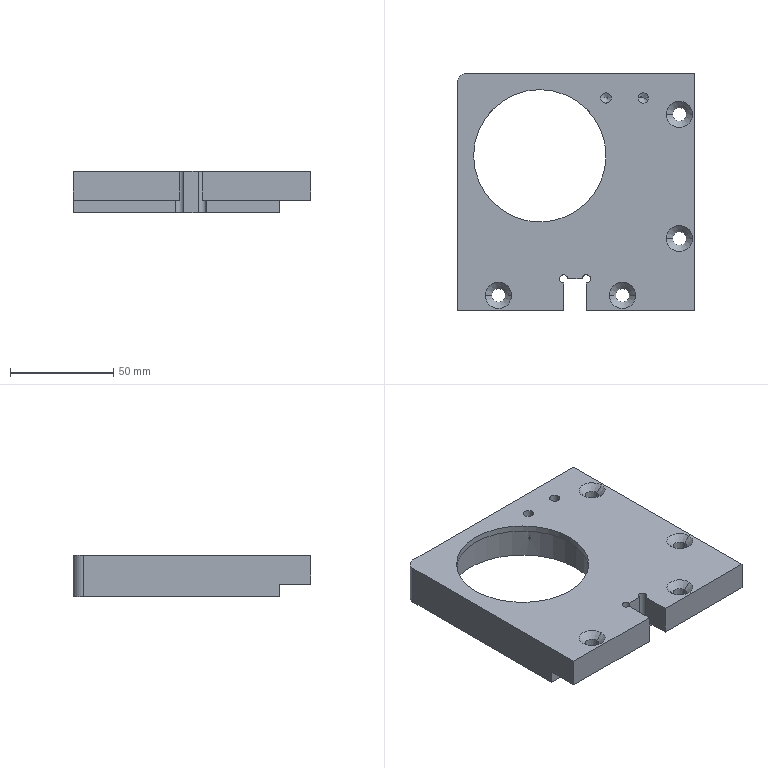Part | SolidWorks | features ICE 5, HoleWzd 3, Extrusion 1, Fillet 1 | 1 solid | 55 faces | box 115 x 115 x 20 mm | volume 159742 mm3 | cylinder 25 | plane 16 | cone 14 | commonest cylinder face diameters 5 x9 6.6 x8 4 x3 64 x2 72 x2 10 x1